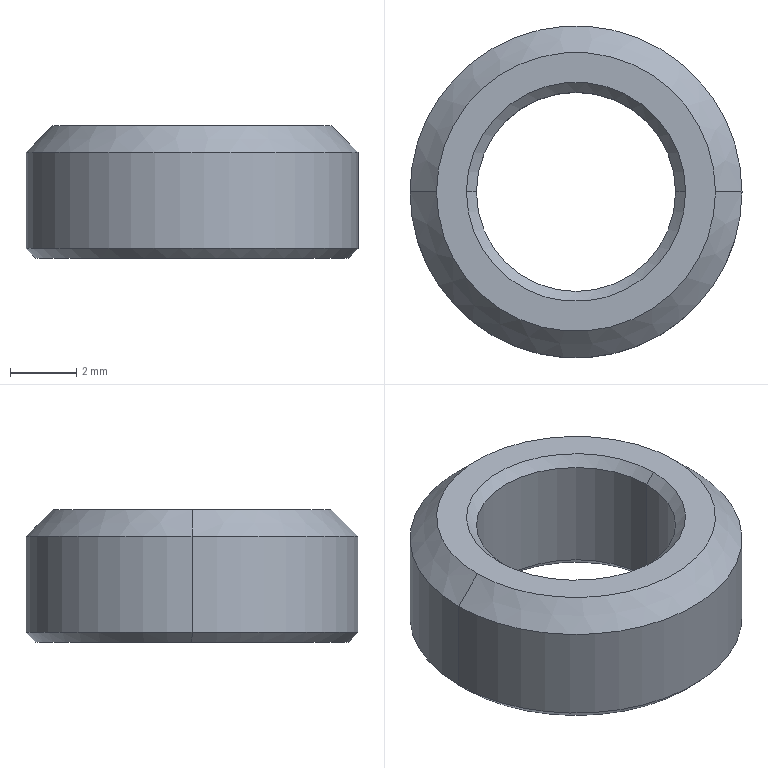Part | SolidWorks | features BaseBody 1 | 1 solid | 14 faces | box 10 x 10 x 4 mm | volume 188.407 mm3 | cone 8 | cylinder 4 | plane 2 | commonest cylinder face diameters 6 x2 10 x2
STEP:
#1=CARTESIAN_POINT('',(4.2,0.,4.));
#2=VERTEX_POINT('',#1);
#3=CARTESIAN_POINT('',(-4.2,0.,4.));
#4=VERTEX_POINT('',#3);
#5=CARTESIAN_POINT('',(0.,0.,4.));
#6=DIRECTION('',(0.,0.,1.));
#7=DIRECTION('',(1.,0.,0.));
#8=AXIS2_PLACEMENT_3D('',#5,#6,#7);
#9=CIRCLE('',#8,4.2);
#10=EDGE_CURVE('',#2,#4,#9,.T.);
#11=ORIENTED_EDGE('',*,*,#10,.F.);
#12=CARTESIAN_POINT('',(5.,0.,3.2));
#13=VERTEX_POINT('',#12);
#14=CARTESIAN_POINT('',(4.2,0.,4.));
#15=DIRECTION('',(0.7071,0.,-0.7071));
#16=VECTOR('',#15,1000.);
#17=LINE('',#14,#16);
#18=EDGE_CURVE('',#2,#13,#17,.T.);
#19=ORIENTED_EDGE('',*,*,#18,.T.);
#20=CARTESIAN_POINT('',(-5.,0.,3.2));
#21=VERTEX_POINT('',#20);
#22=CARTESIAN_POINT('',(0.,0.,3.2));
#23=DIRECTION('',(0.,0.,-1.));
#24=DIRECTION('',(1.,0.,0.));
#25=AXIS2_PLACEMENT_3D('',#22,#23,#24);
#26=CIRCLE('',#25,5.);
#27=EDGE_CURVE('',#21,#13,#26,.T.);
#28=ORIENTED_EDGE('',*,*,#27,.F.);
#29=CARTESIAN_POINT('',(-4.2,0.,4.));
#30=DIRECTION('',(-0.7071,0.,-0.7071));
#31=VECTOR('',#30,1000.);
#32=LINE('',#29,#31);
#33=EDGE_CURVE('',#4,#21,#32,.T.);
#34=ORIENTED_EDGE('',*,*,#33,.F.);
#35=EDGE_LOOP('',(#11,#19,#28,#34));
#36=FACE_OUTER_BOUND('',#35,.T.);
#37=CARTESIAN_POINT('',(0.,0.,4.));
#38=DIRECTION('',(0.,0.,-1.));
#39=DIRECTION('',(-1.,0.,0.));
#40=AXIS2_PLACEMENT_3D('',#37,#38,#39);
#41=CONICAL_SURFACE('',#40,4.2,0.7854);
#42=ADVANCED_FACE('',(#36),#41,.T.);
#43=CARTESIAN_POINT('',(-3.,0.,3.7));
#44=VERTEX_POINT('',#43);
#45=CARTESIAN_POINT('',(3.,0.,3.7));
#46=VERTEX_POINT('',#45);
#47=CARTESIAN_POINT('',(0.,0.,3.7));
#48=DIRECTION('',(0.,0.,1.));
#49=DIRECTION('',(1.,0.,0.));
#50=AXIS2_PLACEMENT_3D('',#47,#48,#49);
#51=CIRCLE('',#50,3.);
#52=EDGE_CURVE('',#44,#46,#51,.T.);
#53=ORIENTED_EDGE('',*,*,#52,.F.);
#54=CARTESIAN_POINT('',(-3.3,0.,4.));
#55=VERTEX_POINT('',#54);
#56=CARTESIAN_POINT('',(-3.,0.,3.7));
#57=DIRECTION('',(-0.7071,0.,0.7071));
#58=VECTOR('',#57,1000.);
#59=LINE('',#56,#58);
#60=EDGE_CURVE('',#44,#55,#59,.T.);
#61=ORIENTED_EDGE('',*,*,#60,.T.);
#62=CARTESIAN_POINT('',(3.3,0.,4.));
#63=VERTEX_POINT('',#62);
#64=CARTESIAN_POINT('',(0.,0.,4.));
#65=DIRECTION('',(0.,0.,-1.));
#66=DIRECTION('',(1.,0.,0.));
#67=AXIS2_PLACEMENT_3D('',#64,#65,#66);
#68=CIRCLE('',#67,3.3);
#69=EDGE_CURVE('',#63,#55,#68,.T.);
#70=ORIENTED_EDGE('',*,*,#69,.F.);
#71=CARTESIAN_POINT('',(3.,0.,3.7));
#72=DIRECTION('',(0.7071,0.,0.7071));
#73=VECTOR('',#72,1000.);
#74=LINE('',#71,#73);
#75=EDGE_CURVE('',#46,#63,#74,.T.);
#76=ORIENTED_EDGE('',*,*,#75,.F.);
#77=EDGE_LOOP('',(#53,#61,#70,#76));
#78=FACE_OUTER_BOUND('',#77,.T.);
#79=CARTESIAN_POINT('',(0.,0.,3.7));
#80=DIRECTION('',(0.,0.,1.));
#81=DIRECTION('',(1.,0.,0.));
#82=AXIS2_PLACEMENT_3D('',#79,#80,#81);
#83=CONICAL_SURFACE('',#82,3.,0.7854);
#84=ADVANCED_FACE('',(#78),#83,.F.);
#85=CARTESIAN_POINT('',(-4.7,0.,0.));
#86=VERTEX_POINT('',#85);
#87=CARTESIAN_POINT('',(4.7,0.,0.));
#88=VERTEX_POINT('',#87);
#89=CARTESIAN_POINT('',(0.,0.,0.));
#90=DIRECTION('',(0.,0.,-1.));
#91=DIRECTION('',(1.,0.,0.));
#92=AXIS2_PLACEMENT_3D('',#89,#90,#91);
#93=CIRCLE('',#92,4.7);
#94=EDGE_CURVE('',#86,#88,#93,.T.);
#95=ORIENTED_EDGE('',*,*,#94,.F.);
#96=CARTESIAN_POINT('',(-5.,0.,0.3));
#97=VERTEX_POINT('',#96);
#98=CARTESIAN_POINT('',(-5.,0.,0.3));
#99=DIRECTION('',(-0.7071,0.,0.7071));
#100=VECTOR('',#99,1000.);
#101=LINE('',#98,#100);
#102=EDGE_CURVE('',#86,#97,#101,.T.);
#103=ORIENTED_EDGE('',*,*,#102,.T.);
#104=CARTESIAN_POINT('',(5.,0.,0.3));
#105=VERTEX_POINT('',#104);
#106=CARTESIAN_POINT('',(0.,0.,0.3));
#107=DIRECTION('',(0.,0.,1.));
#108=DIRECTION('',(1.,0.,0.));
#109=AXIS2_PLACEMENT_3D('',#106,#107,#108);
#110=CIRCLE('',#109,5.);
#111=EDGE_CURVE('',#105,#97,#110,.T.);
#112=ORIENTED_EDGE('',*,*,#111,.F.);
#113=CARTESIAN_POINT('',(5.,0.,0.3));
#114=DIRECTION('',(0.7071,0.,0.7071));
#115=VECTOR('',#114,1000.);
#116=LINE('',#113,#115);
#117=EDGE_CURVE('',#88,#105,#116,.T.);
#118=ORIENTED_EDGE('',*,*,#117,.F.);
#119=EDGE_LOOP('',(#95,#103,#112,#118));
#120=FACE_OUTER_BOUND('',#119,.T.);
#121=CARTESIAN_POINT('',(0.,0.,0.3));
#122=DIRECTION('',(0.,0.,1.));
#123=DIRECTION('',(1.,0.,0.));
#124=AXIS2_PLACEMENT_3D('',#121,#122,#123);
#125=CONICAL_SURFACE('',#124,5.,0.7854);
#126=ADVANCED_FACE('',(#120),#125,.T.);
#127=CARTESIAN_POINT('',(3.,0.,0.3));
#128=VERTEX_POINT('',#127);
#129=CARTESIAN_POINT('',(-3.,0.,0.3));
#130=VERTEX_POINT('',#129);
#131=CARTESIAN_POINT('',(0.,0.,0.3));
#132=DIRECTION('',(0.,0.,-1.));
#133=DIRECTION('',(1.,0.,0.));
#134=AXIS2_PLACEMENT_3D('',#131,#132,#133);
#135=CIRCLE('',#134,3.);
#136=EDGE_CURVE('',#128,#130,#135,.T.);
#137=ORIENTED_EDGE('',*,*,#136,.F.);
#138=CARTESIAN_POINT('',(3.3,0.,0.));
#139=VERTEX_POINT('',#138);
#140=CARTESIAN_POINT('',(3.3,0.,0.));
#141=DIRECTION('',(0.7071,0.,-0.7071));
#142=VECTOR('',#141,1000.);
#143=LINE('',#140,#142);
#144=EDGE_CURVE('',#128,#139,#143,.T.);
#145=ORIENTED_EDGE('',*,*,#144,.T.);
#146=CARTESIAN_POINT('',(-3.3,0.,0.));
#147=VERTEX_POINT('',#146);
#148=CARTESIAN_POINT('',(0.,0.,0.));
#149=DIRECTION('',(0.,0.,1.));
#150=DIRECTION('',(1.,0.,0.));
#151=AXIS2_PLACEMENT_3D('',#148,#149,#150);
#152=CIRCLE('',#151,3.3);
#153=EDGE_CURVE('',#147,#139,#152,.T.);
#154=ORIENTED_EDGE('',*,*,#153,.F.);
#155=CARTESIAN_POINT('',(-3.3,0.,0.));
#156=DIRECTION('',(-0.7071,0.,-0.7071));
#157=VECTOR('',#156,1000.);
#158=LINE('',#155,#157);
#159=EDGE_CURVE('',#130,#147,#158,.T.);
#160=ORIENTED_EDGE('',*,*,#159,.F.);
#161=EDGE_LOOP('',(#137,#145,#154,#160));
#162=FACE_OUTER_BOUND('',#161,.T.);
#163=CARTESIAN_POINT('',(0.,0.,0.));
#164=DIRECTION('',(0.,0.,-1.));
#165=DIRECTION('',(-1.,0.,0.));
#166=AXIS2_PLACEMENT_3D('',#163,#164,#165);
#167=CONICAL_SURFACE('',#166,3.3,0.7854);
#168=ADVANCED_FACE('',(#162),#167,.F.);
#169=ORIENTED_EDGE('',*,*,#52,.T.);
#170=CARTESIAN_POINT('',(3.,0.,4.));
#171=DIRECTION('',(0.,0.,-1.));
#172=VECTOR('',#171,1000.);
#173=LINE('',#170,#172);
#174=EDGE_CURVE('',#46,#128,#173,.T.);
#175=ORIENTED_EDGE('',*,*,#174,.T.);
#176=ORIENTED_EDGE('',*,*,#136,.T.);
#177=CARTESIAN_POINT('',(-3.,0.,4.));
#178=DIRECTION('',(0.,0.,-1.));
#179=VECTOR('',#178,1000.);
#180=LINE('',#177,#179);
#181=EDGE_CURVE('',#44,#130,#180,.T.);
#182=ORIENTED_EDGE('',*,*,#181,.F.);
#183=EDGE_LOOP('',(#169,#175,#176,#182));
#184=FACE_OUTER_BOUND('',#183,.T.);
#185=CARTESIAN_POINT('',(0.,0.,4.));
#186=DIRECTION('',(0.,0.,-1.));
#187=DIRECTION('',(-1.,0.,0.));
#188=AXIS2_PLACEMENT_3D('',#185,#186,#187);
#189=CYLINDRICAL_SURFACE('',#188,3.);
#190=ADVANCED_FACE('',(#184),#189,.F.);
#191=ORIENTED_EDGE('',*,*,#27,.T.);
#192=CARTESIAN_POINT('',(5.,0.,4.));
#193=DIRECTION('',(0.,0.,-1.));
#194=VECTOR('',#193,1000.);
#195=LINE('',#192,#194);
#196=EDGE_CURVE('',#13,#105,#195,.T.);
#197=ORIENTED_EDGE('',*,*,#196,.T.);
#198=ORIENTED_EDGE('',*,*,#111,.T.);
#199=CARTESIAN_POINT('',(-5.,0.,4.));
#200=DIRECTION('',(0.,0.,-1.));
#201=VECTOR('',#200,1000.);
#202=LINE('',#199,#201);
#203=EDGE_CURVE('',#21,#97,#202,.T.);
#204=ORIENTED_EDGE('',*,*,#203,.F.);
#205=EDGE_LOOP('',(#191,#197,#198,#204));
#206=FACE_OUTER_BOUND('',#205,.T.);
#207=CARTESIAN_POINT('',(0.,0.,4.));
#208=DIRECTION('',(0.,0.,-1.));
#209=DIRECTION('',(-1.,0.,0.));
#210=AXIS2_PLACEMENT_3D('',#207,#208,#209);
#211=CYLINDRICAL_SURFACE('',#210,5.);
#212=ADVANCED_FACE('',(#206),#211,.T.);
#213=ORIENTED_EDGE('',*,*,#153,.T.);
#214=CARTESIAN_POINT('',(0.,0.,0.));
#215=DIRECTION('',(0.,0.,1.));
#216=DIRECTION('',(1.,0.,0.));
#217=AXIS2_PLACEMENT_3D('',#214,#215,#216);
#218=CIRCLE('',#217,3.3);
#219=EDGE_CURVE('',#139,#147,#218,.T.);
#220=ORIENTED_EDGE('',*,*,#219,.T.);
#221=EDGE_LOOP('',(#213,#220));
#222=FACE_BOUND('',#221,.T.);
#223=CARTESIAN_POINT('',(0.,0.,0.));
#224=DIRECTION('',(0.,0.,-1.));
#225=DIRECTION('',(1.,0.,0.));
#226=AXIS2_PLACEMENT_3D('',#223,#224,#225);
#227=CIRCLE('',#226,4.7);
#228=EDGE_CURVE('',#88,#86,#227,.T.);
#229=ORIENTED_EDGE('',*,*,#228,.T.);
#230=ORIENTED_EDGE('',*,*,#94,.T.);
#231=EDGE_LOOP('',(#229,#230));
#232=FACE_OUTER_BOUND('',#231,.T.);
#233=CARTESIAN_POINT('',(0.,0.,0.));
#234=DIRECTION('',(0.,0.,1.));
#235=DIRECTION('',(1.,0.,0.));
#236=AXIS2_PLACEMENT_3D('',#233,#234,#235);
#237=PLANE('',#236);
#238=ADVANCED_FACE('',(#222,#232),#237,.F.);
#239=ORIENTED_EDGE('',*,*,#69,.T.);
#240=CARTESIAN_POINT('',(0.,0.,4.));
#241=DIRECTION('',(0.,0.,-1.));
#242=DIRECTION('',(1.,0.,0.));
#243=AXIS2_PLACEMENT_3D('',#240,#241,#242);
#244=CIRCLE('',#243,3.3);
#245=EDGE_CURVE('',#55,#63,#244,.T.);
#246=ORIENTED_EDGE('',*,*,#245,.T.);
#247=EDGE_LOOP('',(#239,#246));
#248=FACE_BOUND('',#247,.T.);
#249=CARTESIAN_POINT('',(0.,0.,4.));
#250=DIRECTION('',(0.,0.,1.));
#251=DIRECTION('',(1.,0.,0.));
#252=AXIS2_PLACEMENT_3D('',#249,#250,#251);
#253=CIRCLE('',#252,4.2);
#254=EDGE_CURVE('',#4,#2,#253,.T.);
#255=ORIENTED_EDGE('',*,*,#254,.T.);
#256=ORIENTED_EDGE('',*,*,#10,.T.);
#257=EDGE_LOOP('',(#255,#256));
#258=FACE_OUTER_BOUND('',#257,.T.);
#259=CARTESIAN_POINT('',(0.,0.,4.));
#260=DIRECTION('',(0.,0.,1.));
#261=DIRECTION('',(1.,0.,0.));
#262=AXIS2_PLACEMENT_3D('',#259,#260,#261);
#263=PLANE('',#262);
#264=ADVANCED_FACE('',(#248,#258),#263,.T.);
#265=ORIENTED_EDGE('',*,*,#196,.F.);
#266=CARTESIAN_POINT('',(0.,0.,3.2));
#267=DIRECTION('',(0.,0.,-1.));
#268=DIRECTION('',(1.,0.,0.));
#269=AXIS2_PLACEMENT_3D('',#266,#267,#268);
#270=CIRCLE('',#269,5.);
#271=EDGE_CURVE('',#13,#21,#270,.T.);
#272=ORIENTED_EDGE('',*,*,#271,.T.);
#273=ORIENTED_EDGE('',*,*,#203,.T.);
#274=CARTESIAN_POINT('',(0.,0.,0.3));
#275=DIRECTION('',(0.,0.,1.));
#276=DIRECTION('',(1.,0.,0.));
#277=AXIS2_PLACEMENT_3D('',#274,#275,#276);
#278=CIRCLE('',#277,5.);
#279=EDGE_CURVE('',#97,#105,#278,.T.);
#280=ORIENTED_EDGE('',*,*,#279,.T.);
#281=EDGE_LOOP('',(#265,#272,#273,#280));
#282=FACE_OUTER_BOUND('',#281,.T.);
#283=CARTESIAN_POINT('',(0.,0.,4.));
#284=DIRECTION('',(0.,0.,-1.));
#285=DIRECTION('',(-1.,0.,0.));
#286=AXIS2_PLACEMENT_3D('',#283,#284,#285);
#287=CYLINDRICAL_SURFACE('',#286,5.);
#288=ADVANCED_FACE('',(#282),#287,.T.);
#289=ORIENTED_EDGE('',*,*,#174,.F.);
#290=CARTESIAN_POINT('',(0.,0.,3.7));
#291=DIRECTION('',(0.,0.,1.));
#292=DIRECTION('',(1.,0.,0.));
#293=AXIS2_PLACEMENT_3D('',#290,#291,#292);
#294=CIRCLE('',#293,3.);
#295=EDGE_CURVE('',#46,#44,#294,.T.);
#296=ORIENTED_EDGE('',*,*,#295,.T.);
#297=ORIENTED_EDGE('',*,*,#181,.T.);
#298=CARTESIAN_POINT('',(0.,0.,0.3));
#299=DIRECTION('',(0.,0.,-1.));
#300=DIRECTION('',(1.,0.,0.));
#301=AXIS2_PLACEMENT_3D('',#298,#299,#300);
#302=CIRCLE('',#301,3.);
#303=EDGE_CURVE('',#130,#128,#302,.T.);
#304=ORIENTED_EDGE('',*,*,#303,.T.);
#305=EDGE_LOOP('',(#289,#296,#297,#304));
#306=FACE_OUTER_BOUND('',#305,.T.);
#307=CARTESIAN_POINT('',(0.,0.,4.));
#308=DIRECTION('',(0.,0.,-1.));
#309=DIRECTION('',(-1.,0.,0.));
#310=AXIS2_PLACEMENT_3D('',#307,#308,#309);
#311=CYLINDRICAL_SURFACE('',#310,3.);
#312=ADVANCED_FACE('',(#306),#311,.F.);
#313=ORIENTED_EDGE('',*,*,#144,.F.);
#314=ORIENTED_EDGE('',*,*,#303,.F.);
#315=ORIENTED_EDGE('',*,*,#159,.T.);
#316=ORIENTED_EDGE('',*,*,#219,.F.);
#317=EDGE_LOOP('',(#313,#314,#315,#316));
#318=FACE_OUTER_BOUND('',#317,.T.);
#319=CARTESIAN_POINT('',(0.,0.,0.));
#320=DIRECTION('',(0.,0.,-1.));
#321=DIRECTION('',(-1.,0.,0.));
#322=AXIS2_PLACEMENT_3D('',#319,#320,#321);
#323=CONICAL_SURFACE('',#322,3.3,0.7854);
#324=ADVANCED_FACE('',(#318),#323,.F.);
#325=ORIENTED_EDGE('',*,*,#102,.F.);
#326=ORIENTED_EDGE('',*,*,#228,.F.);
#327=ORIENTED_EDGE('',*,*,#117,.T.);
#328=ORIENTED_EDGE('',*,*,#279,.F.);
#329=EDGE_LOOP('',(#325,#326,#327,#328));
#330=FACE_OUTER_BOUND('',#329,.T.);
#331=CARTESIAN_POINT('',(0.,0.,0.3));
#332=DIRECTION('',(0.,0.,1.));
#333=DIRECTION('',(1.,0.,0.));
#334=AXIS2_PLACEMENT_3D('',#331,#332,#333);
#335=CONICAL_SURFACE('',#334,5.,0.7854);
#336=ADVANCED_FACE('',(#330),#335,.T.);
#337=ORIENTED_EDGE('',*,*,#60,.F.);
#338=ORIENTED_EDGE('',*,*,#295,.F.);
#339=ORIENTED_EDGE('',*,*,#75,.T.);
#340=ORIENTED_EDGE('',*,*,#245,.F.);
#341=EDGE_LOOP('',(#337,#338,#339,#340));
#342=FACE_OUTER_BOUND('',#341,.T.);
#343=CARTESIAN_POINT('',(0.,0.,3.7));
#344=DIRECTION('',(0.,0.,1.));
#345=DIRECTION('',(1.,0.,0.));
#346=AXIS2_PLACEMENT_3D('',#343,#344,#345);
#347=CONICAL_SURFACE('',#346,3.,0.7854);
#348=ADVANCED_FACE('',(#342),#347,.F.);
#349=ORIENTED_EDGE('',*,*,#18,.F.);
#350=ORIENTED_EDGE('',*,*,#254,.F.);
#351=ORIENTED_EDGE('',*,*,#33,.T.);
#352=ORIENTED_EDGE('',*,*,#271,.F.);
#353=EDGE_LOOP('',(#349,#350,#351,#352));
#354=FACE_OUTER_BOUND('',#353,.T.);
#355=CARTESIAN_POINT('',(0.,0.,4.));
#356=DIRECTION('',(0.,0.,-1.));
#357=DIRECTION('',(-1.,0.,0.));
#358=AXIS2_PLACEMENT_3D('',#355,#356,#357);
#359=CONICAL_SURFACE('',#358,4.2,0.7854);
#360=ADVANCED_FACE('',(#354),#359,.T.);
#361=CLOSED_SHELL('',(#42,#84,#126,#168,#190,#212,#238,#264,#288,#312,#324,#336,#348,#360));
#362=MANIFOLD_SOLID_BREP('',#361);
#363=CARTESIAN_POINT('',(0.,0.,0.));
#364=DIRECTION('',(0.,0.,1.));
#365=DIRECTION('',(1.,0.,0.));
#366=AXIS2_PLACEMENT_3D('',#363,#364,#365);
#367=(LENGTH_UNIT()NAMED_UNIT(*)SI_UNIT(.MILLI.,.METRE.));
#368=UNCERTAINTY_MEASURE_WITH_UNIT(LENGTH_MEASURE(0.00001),#367,'','');
#369=(NAMED_UNIT(*)PLANE_ANGLE_UNIT()SI_UNIT($,.RADIAN.));
#370=(NAMED_UNIT(*)SI_UNIT($,.STERADIAN.)SOLID_ANGLE_UNIT());
#371=(GEOMETRIC_REPRESENTATION_CONTEXT(3)GLOBAL_UNCERTAINTY_ASSIGNED_CONTEXT((#368))GLOBAL_UNIT_ASSIGNED_CONTEXT((#367,#369,#370))REPRESENTATION_CONTEXT('',''));
#372=ADVANCED_BREP_SHAPE_REPRESENTATION('',(#362,#366),#371);